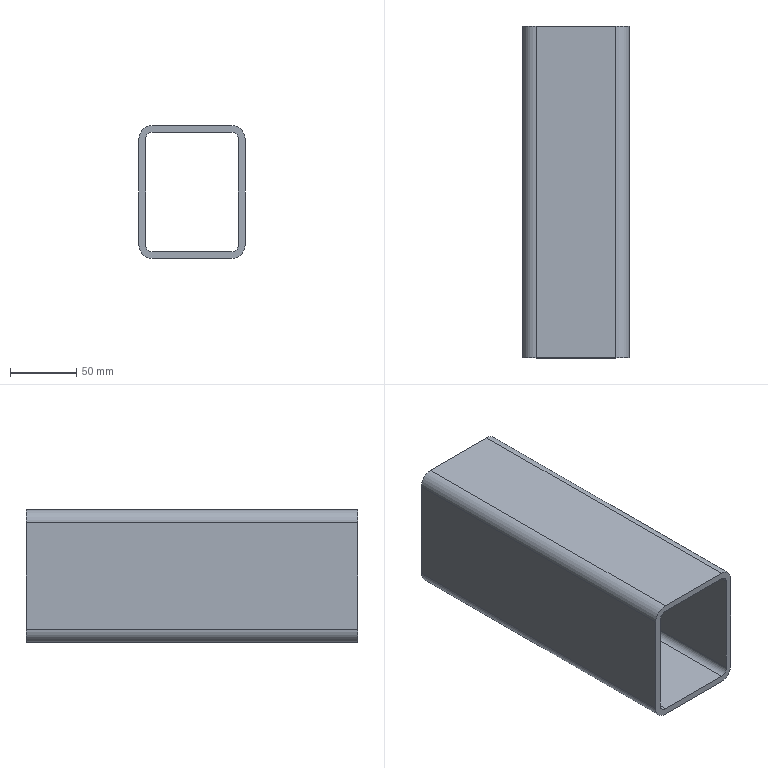Part | SolidWorks | features WeldMemberFeat 1, WeldmentFeature 1 | 1 solid | 18 faces | box 80 x 250 x 100 mm | volume 408905 mm3 | plane 10 | cylinder 8 | commonest cylinder face diameters 10 x4 20 x4
STEP:
#1=CARTESIAN_POINT('',(-40.,0.,40.));
#2=VERTEX_POINT('',#1);
#3=CARTESIAN_POINT('',(-30.,0.,50.));
#4=VERTEX_POINT('',#3);
#5=CARTESIAN_POINT('',(-30.,0.,40.));
#6=DIRECTION('',(0.,1.,0.));
#7=DIRECTION('',(0.,0.,1.));
#8=AXIS2_PLACEMENT_3D('',#5,#6,#7);
#9=CIRCLE('',#8,10.);
#10=EDGE_CURVE('',#2,#4,#9,.T.);
#11=ORIENTED_EDGE('',*,*,#10,.T.);
#12=CARTESIAN_POINT('',(-30.,250.,50.));
#13=VERTEX_POINT('',#12);
#14=CARTESIAN_POINT('',(-30.,250.,50.));
#15=DIRECTION('',(0.,-1.,0.));
#16=VECTOR('',#15,1000.);
#17=LINE('',#14,#16);
#18=EDGE_CURVE('',#13,#4,#17,.T.);
#19=ORIENTED_EDGE('',*,*,#18,.F.);
#20=CARTESIAN_POINT('',(-40.,250.,40.));
#21=VERTEX_POINT('',#20);
#22=CARTESIAN_POINT('',(-30.,250.,40.));
#23=DIRECTION('',(0.,1.,0.));
#24=DIRECTION('',(0.,0.,1.));
#25=AXIS2_PLACEMENT_3D('',#22,#23,#24);
#26=CIRCLE('',#25,10.);
#27=EDGE_CURVE('',#21,#13,#26,.T.);
#28=ORIENTED_EDGE('',*,*,#27,.F.);
#29=CARTESIAN_POINT('',(-40.,250.,40.));
#30=DIRECTION('',(0.,-1.,0.));
#31=VECTOR('',#30,1000.);
#32=LINE('',#29,#31);
#33=EDGE_CURVE('',#21,#2,#32,.T.);
#34=ORIENTED_EDGE('',*,*,#33,.T.);
#35=EDGE_LOOP('',(#11,#19,#28,#34));
#36=FACE_OUTER_BOUND('',#35,.T.);
#37=CARTESIAN_POINT('',(-30.,250.,40.));
#38=DIRECTION('',(0.,-1.,0.));
#39=DIRECTION('',(0.,0.,-1.));
#40=AXIS2_PLACEMENT_3D('',#37,#38,#39);
#41=CYLINDRICAL_SURFACE('',#40,10.);
#42=ADVANCED_FACE('',(#36),#41,.T.);
#43=CARTESIAN_POINT('',(30.,0.,50.));
#44=VERTEX_POINT('',#43);
#45=CARTESIAN_POINT('',(-30.,0.,50.));
#46=DIRECTION('',(1.,0.,0.));
#47=VECTOR('',#46,1000.);
#48=LINE('',#45,#47);
#49=EDGE_CURVE('',#4,#44,#48,.T.);
#50=ORIENTED_EDGE('',*,*,#49,.T.);
#51=CARTESIAN_POINT('',(30.,250.,50.));
#52=VERTEX_POINT('',#51);
#53=CARTESIAN_POINT('',(30.,250.,50.));
#54=DIRECTION('',(0.,-1.,0.));
#55=VECTOR('',#54,1000.);
#56=LINE('',#53,#55);
#57=EDGE_CURVE('',#52,#44,#56,.T.);
#58=ORIENTED_EDGE('',*,*,#57,.F.);
#59=CARTESIAN_POINT('',(-30.,250.,50.));
#60=DIRECTION('',(1.,0.,0.));
#61=VECTOR('',#60,1000.);
#62=LINE('',#59,#61);
#63=EDGE_CURVE('',#13,#52,#62,.T.);
#64=ORIENTED_EDGE('',*,*,#63,.F.);
#65=ORIENTED_EDGE('',*,*,#18,.T.);
#66=EDGE_LOOP('',(#50,#58,#64,#65));
#67=FACE_OUTER_BOUND('',#66,.T.);
#68=CARTESIAN_POINT('',(-30.,250.,50.));
#69=DIRECTION('',(0.,0.,-1.));
#70=DIRECTION('',(-1.,0.,0.));
#71=AXIS2_PLACEMENT_3D('',#68,#69,#70);
#72=PLANE('',#71);
#73=ADVANCED_FACE('',(#67),#72,.F.);
#74=CARTESIAN_POINT('',(40.,0.,40.));
#75=VERTEX_POINT('',#74);
#76=CARTESIAN_POINT('',(30.,0.,40.));
#77=DIRECTION('',(0.,1.,0.));
#78=DIRECTION('',(0.,0.,1.));
#79=AXIS2_PLACEMENT_3D('',#76,#77,#78);
#80=CIRCLE('',#79,10.);
#81=EDGE_CURVE('',#44,#75,#80,.T.);
#82=ORIENTED_EDGE('',*,*,#81,.T.);
#83=CARTESIAN_POINT('',(40.,250.,40.));
#84=VERTEX_POINT('',#83);
#85=CARTESIAN_POINT('',(40.,250.,40.));
#86=DIRECTION('',(0.,-1.,0.));
#87=VECTOR('',#86,1000.);
#88=LINE('',#85,#87);
#89=EDGE_CURVE('',#84,#75,#88,.T.);
#90=ORIENTED_EDGE('',*,*,#89,.F.);
#91=CARTESIAN_POINT('',(30.,250.,40.));
#92=DIRECTION('',(0.,1.,0.));
#93=DIRECTION('',(0.,0.,1.));
#94=AXIS2_PLACEMENT_3D('',#91,#92,#93);
#95=CIRCLE('',#94,10.);
#96=EDGE_CURVE('',#52,#84,#95,.T.);
#97=ORIENTED_EDGE('',*,*,#96,.F.);
#98=ORIENTED_EDGE('',*,*,#57,.T.);
#99=EDGE_LOOP('',(#82,#90,#97,#98));
#100=FACE_OUTER_BOUND('',#99,.T.);
#101=CARTESIAN_POINT('',(30.,250.,40.));
#102=DIRECTION('',(0.,-1.,0.));
#103=DIRECTION('',(0.,0.,-1.));
#104=AXIS2_PLACEMENT_3D('',#101,#102,#103);
#105=CYLINDRICAL_SURFACE('',#104,10.);
#106=ADVANCED_FACE('',(#100),#105,.T.);
#107=CARTESIAN_POINT('',(40.,0.,-40.));
#108=VERTEX_POINT('',#107);
#109=CARTESIAN_POINT('',(40.,0.,-40.));
#110=DIRECTION('',(0.,0.,-1.));
#111=VECTOR('',#110,1000.);
#112=LINE('',#109,#111);
#113=EDGE_CURVE('',#75,#108,#112,.T.);
#114=ORIENTED_EDGE('',*,*,#113,.T.);
#115=CARTESIAN_POINT('',(40.,250.,-40.));
#116=VERTEX_POINT('',#115);
#117=CARTESIAN_POINT('',(40.,250.,-40.));
#118=DIRECTION('',(0.,-1.,0.));
#119=VECTOR('',#118,1000.);
#120=LINE('',#117,#119);
#121=EDGE_CURVE('',#116,#108,#120,.T.);
#122=ORIENTED_EDGE('',*,*,#121,.F.);
#123=CARTESIAN_POINT('',(40.,250.,-40.));
#124=DIRECTION('',(0.,0.,-1.));
#125=VECTOR('',#124,1000.);
#126=LINE('',#123,#125);
#127=EDGE_CURVE('',#84,#116,#126,.T.);
#128=ORIENTED_EDGE('',*,*,#127,.F.);
#129=ORIENTED_EDGE('',*,*,#89,.T.);
#130=EDGE_LOOP('',(#114,#122,#128,#129));
#131=FACE_OUTER_BOUND('',#130,.T.);
#132=CARTESIAN_POINT('',(40.,250.,-40.));
#133=DIRECTION('',(-1.,0.,0.));
#134=DIRECTION('',(0.,0.,1.));
#135=AXIS2_PLACEMENT_3D('',#132,#133,#134);
#136=PLANE('',#135);
#137=ADVANCED_FACE('',(#131),#136,.F.);
#138=CARTESIAN_POINT('',(30.,0.,-50.));
#139=VERTEX_POINT('',#138);
#140=CARTESIAN_POINT('',(30.,0.,-40.));
#141=DIRECTION('',(0.,1.,0.));
#142=DIRECTION('',(0.,0.,1.));
#143=AXIS2_PLACEMENT_3D('',#140,#141,#142);
#144=CIRCLE('',#143,10.);
#145=EDGE_CURVE('',#108,#139,#144,.T.);
#146=ORIENTED_EDGE('',*,*,#145,.T.);
#147=CARTESIAN_POINT('',(30.,250.,-50.));
#148=VERTEX_POINT('',#147);
#149=CARTESIAN_POINT('',(30.,250.,-50.));
#150=DIRECTION('',(0.,-1.,0.));
#151=VECTOR('',#150,1000.);
#152=LINE('',#149,#151);
#153=EDGE_CURVE('',#148,#139,#152,.T.);
#154=ORIENTED_EDGE('',*,*,#153,.F.);
#155=CARTESIAN_POINT('',(30.,250.,-40.));
#156=DIRECTION('',(0.,1.,0.));
#157=DIRECTION('',(0.,0.,1.));
#158=AXIS2_PLACEMENT_3D('',#155,#156,#157);
#159=CIRCLE('',#158,10.);
#160=EDGE_CURVE('',#116,#148,#159,.T.);
#161=ORIENTED_EDGE('',*,*,#160,.F.);
#162=ORIENTED_EDGE('',*,*,#121,.T.);
#163=EDGE_LOOP('',(#146,#154,#161,#162));
#164=FACE_OUTER_BOUND('',#163,.T.);
#165=CARTESIAN_POINT('',(30.,250.,-40.));
#166=DIRECTION('',(0.,-1.,0.));
#167=DIRECTION('',(0.,0.,-1.));
#168=AXIS2_PLACEMENT_3D('',#165,#166,#167);
#169=CYLINDRICAL_SURFACE('',#168,10.);
#170=ADVANCED_FACE('',(#164),#169,.T.);
#171=CARTESIAN_POINT('',(-30.,0.,-50.));
#172=VERTEX_POINT('',#171);
#173=CARTESIAN_POINT('',(30.,0.,-50.));
#174=DIRECTION('',(-1.,0.,0.));
#175=VECTOR('',#174,1000.);
#176=LINE('',#173,#175);
#177=EDGE_CURVE('',#139,#172,#176,.T.);
#178=ORIENTED_EDGE('',*,*,#177,.T.);
#179=CARTESIAN_POINT('',(-30.,250.,-50.));
#180=VERTEX_POINT('',#179);
#181=CARTESIAN_POINT('',(-30.,250.,-50.));
#182=DIRECTION('',(0.,-1.,0.));
#183=VECTOR('',#182,1000.);
#184=LINE('',#181,#183);
#185=EDGE_CURVE('',#180,#172,#184,.T.);
#186=ORIENTED_EDGE('',*,*,#185,.F.);
#187=CARTESIAN_POINT('',(30.,250.,-50.));
#188=DIRECTION('',(-1.,0.,0.));
#189=VECTOR('',#188,1000.);
#190=LINE('',#187,#189);
#191=EDGE_CURVE('',#148,#180,#190,.T.);
#192=ORIENTED_EDGE('',*,*,#191,.F.);
#193=ORIENTED_EDGE('',*,*,#153,.T.);
#194=EDGE_LOOP('',(#178,#186,#192,#193));
#195=FACE_OUTER_BOUND('',#194,.T.);
#196=CARTESIAN_POINT('',(30.,250.,-50.));
#197=DIRECTION('',(0.,0.,1.));
#198=DIRECTION('',(1.,0.,0.));
#199=AXIS2_PLACEMENT_3D('',#196,#197,#198);
#200=PLANE('',#199);
#201=ADVANCED_FACE('',(#195),#200,.F.);
#202=CARTESIAN_POINT('',(-40.,0.,-40.));
#203=VERTEX_POINT('',#202);
#204=CARTESIAN_POINT('',(-30.,0.,-40.));
#205=DIRECTION('',(0.,1.,0.));
#206=DIRECTION('',(0.,0.,1.));
#207=AXIS2_PLACEMENT_3D('',#204,#205,#206);
#208=CIRCLE('',#207,10.);
#209=EDGE_CURVE('',#172,#203,#208,.T.);
#210=ORIENTED_EDGE('',*,*,#209,.T.);
#211=CARTESIAN_POINT('',(-40.,250.,-40.));
#212=VERTEX_POINT('',#211);
#213=CARTESIAN_POINT('',(-40.,250.,-40.));
#214=DIRECTION('',(0.,-1.,0.));
#215=VECTOR('',#214,1000.);
#216=LINE('',#213,#215);
#217=EDGE_CURVE('',#212,#203,#216,.T.);
#218=ORIENTED_EDGE('',*,*,#217,.F.);
#219=CARTESIAN_POINT('',(-30.,250.,-40.));
#220=DIRECTION('',(0.,1.,0.));
#221=DIRECTION('',(0.,0.,1.));
#222=AXIS2_PLACEMENT_3D('',#219,#220,#221);
#223=CIRCLE('',#222,10.);
#224=EDGE_CURVE('',#180,#212,#223,.T.);
#225=ORIENTED_EDGE('',*,*,#224,.F.);
#226=ORIENTED_EDGE('',*,*,#185,.T.);
#227=EDGE_LOOP('',(#210,#218,#225,#226));
#228=FACE_OUTER_BOUND('',#227,.T.);
#229=CARTESIAN_POINT('',(-30.,250.,-40.));
#230=DIRECTION('',(0.,-1.,0.));
#231=DIRECTION('',(0.,0.,-1.));
#232=AXIS2_PLACEMENT_3D('',#229,#230,#231);
#233=CYLINDRICAL_SURFACE('',#232,10.);
#234=ADVANCED_FACE('',(#228),#233,.T.);
#235=CARTESIAN_POINT('',(30.,0.,45.));
#236=VERTEX_POINT('',#235);
#237=CARTESIAN_POINT('',(35.,0.,40.));
#238=VERTEX_POINT('',#237);
#239=CARTESIAN_POINT('',(30.,0.,40.));
#240=DIRECTION('',(0.,1.,0.));
#241=DIRECTION('',(0.,0.,1.));
#242=AXIS2_PLACEMENT_3D('',#239,#240,#241);
#243=CIRCLE('',#242,5.);
#244=EDGE_CURVE('',#236,#238,#243,.T.);
#245=ORIENTED_EDGE('',*,*,#244,.F.);
#246=CARTESIAN_POINT('',(30.,250.,45.));
#247=VERTEX_POINT('',#246);
#248=CARTESIAN_POINT('',(30.,250.,45.));
#249=DIRECTION('',(0.,-1.,0.));
#250=VECTOR('',#249,1000.);
#251=LINE('',#248,#250);
#252=EDGE_CURVE('',#247,#236,#251,.T.);
#253=ORIENTED_EDGE('',*,*,#252,.F.);
#254=CARTESIAN_POINT('',(35.,250.,40.));
#255=VERTEX_POINT('',#254);
#256=CARTESIAN_POINT('',(30.,250.,40.));
#257=DIRECTION('',(0.,1.,0.));
#258=DIRECTION('',(0.,0.,1.));
#259=AXIS2_PLACEMENT_3D('',#256,#257,#258);
#260=CIRCLE('',#259,5.);
#261=EDGE_CURVE('',#247,#255,#260,.T.);
#262=ORIENTED_EDGE('',*,*,#261,.T.);
#263=CARTESIAN_POINT('',(35.,250.,40.));
#264=DIRECTION('',(0.,-1.,0.));
#265=VECTOR('',#264,1000.);
#266=LINE('',#263,#265);
#267=EDGE_CURVE('',#255,#238,#266,.T.);
#268=ORIENTED_EDGE('',*,*,#267,.T.);
#269=EDGE_LOOP('',(#245,#253,#262,#268));
#270=FACE_OUTER_BOUND('',#269,.T.);
#271=CARTESIAN_POINT('',(30.,250.,40.));
#272=DIRECTION('',(0.,-1.,0.));
#273=DIRECTION('',(0.,0.,-1.));
#274=AXIS2_PLACEMENT_3D('',#271,#272,#273);
#275=CYLINDRICAL_SURFACE('',#274,5.);
#276=ADVANCED_FACE('',(#270),#275,.F.);
#277=CARTESIAN_POINT('',(-30.,0.,45.));
#278=VERTEX_POINT('',#277);
#279=CARTESIAN_POINT('',(-30.,0.,45.));
#280=DIRECTION('',(1.,0.,0.));
#281=VECTOR('',#280,1000.);
#282=LINE('',#279,#281);
#283=EDGE_CURVE('',#278,#236,#282,.T.);
#284=ORIENTED_EDGE('',*,*,#283,.F.);
#285=CARTESIAN_POINT('',(-30.,250.,45.));
#286=VERTEX_POINT('',#285);
#287=CARTESIAN_POINT('',(-30.,250.,45.));
#288=DIRECTION('',(0.,-1.,0.));
#289=VECTOR('',#288,1000.);
#290=LINE('',#287,#289);
#291=EDGE_CURVE('',#286,#278,#290,.T.);
#292=ORIENTED_EDGE('',*,*,#291,.F.);
#293=CARTESIAN_POINT('',(-30.,250.,45.));
#294=DIRECTION('',(1.,0.,0.));
#295=VECTOR('',#294,1000.);
#296=LINE('',#293,#295);
#297=EDGE_CURVE('',#286,#247,#296,.T.);
#298=ORIENTED_EDGE('',*,*,#297,.T.);
#299=ORIENTED_EDGE('',*,*,#252,.T.);
#300=EDGE_LOOP('',(#284,#292,#298,#299));
#301=FACE_OUTER_BOUND('',#300,.T.);
#302=CARTESIAN_POINT('',(-30.,250.,45.));
#303=DIRECTION('',(0.,0.,-1.));
#304=DIRECTION('',(-1.,0.,0.));
#305=AXIS2_PLACEMENT_3D('',#302,#303,#304);
#306=PLANE('',#305);
#307=ADVANCED_FACE('',(#301),#306,.T.);
#308=CARTESIAN_POINT('',(-35.,0.,40.));
#309=VERTEX_POINT('',#308);
#310=CARTESIAN_POINT('',(-30.,0.,40.));
#311=DIRECTION('',(0.,1.,0.));
#312=DIRECTION('',(0.,0.,1.));
#313=AXIS2_PLACEMENT_3D('',#310,#311,#312);
#314=CIRCLE('',#313,5.);
#315=EDGE_CURVE('',#309,#278,#314,.T.);
#316=ORIENTED_EDGE('',*,*,#315,.F.);
#317=CARTESIAN_POINT('',(-35.,250.,40.));
#318=VERTEX_POINT('',#317);
#319=CARTESIAN_POINT('',(-35.,250.,40.));
#320=DIRECTION('',(0.,-1.,0.));
#321=VECTOR('',#320,1000.);
#322=LINE('',#319,#321);
#323=EDGE_CURVE('',#318,#309,#322,.T.);
#324=ORIENTED_EDGE('',*,*,#323,.F.);
#325=CARTESIAN_POINT('',(-30.,250.,40.));
#326=DIRECTION('',(0.,1.,0.));
#327=DIRECTION('',(0.,0.,1.));
#328=AXIS2_PLACEMENT_3D('',#325,#326,#327);
#329=CIRCLE('',#328,5.);
#330=EDGE_CURVE('',#318,#286,#329,.T.);
#331=ORIENTED_EDGE('',*,*,#330,.T.);
#332=ORIENTED_EDGE('',*,*,#291,.T.);
#333=EDGE_LOOP('',(#316,#324,#331,#332));
#334=FACE_OUTER_BOUND('',#333,.T.);
#335=CARTESIAN_POINT('',(-30.,250.,40.));
#336=DIRECTION('',(0.,-1.,0.));
#337=DIRECTION('',(0.,0.,-1.));
#338=AXIS2_PLACEMENT_3D('',#335,#336,#337);
#339=CYLINDRICAL_SURFACE('',#338,5.);
#340=ADVANCED_FACE('',(#334),#339,.F.);
#341=CARTESIAN_POINT('',(-35.,0.,-40.));
#342=VERTEX_POINT('',#341);
#343=CARTESIAN_POINT('',(-35.,0.,40.));
#344=DIRECTION('',(0.,0.,1.));
#345=VECTOR('',#344,1000.);
#346=LINE('',#343,#345);
#347=EDGE_CURVE('',#342,#309,#346,.T.);
#348=ORIENTED_EDGE('',*,*,#347,.F.);
#349=CARTESIAN_POINT('',(-35.,250.,-40.));
#350=VERTEX_POINT('',#349);
#351=CARTESIAN_POINT('',(-35.,250.,-40.));
#352=DIRECTION('',(0.,-1.,0.));
#353=VECTOR('',#352,1000.);
#354=LINE('',#351,#353);
#355=EDGE_CURVE('',#350,#342,#354,.T.);
#356=ORIENTED_EDGE('',*,*,#355,.F.);
#357=CARTESIAN_POINT('',(-35.,250.,40.));
#358=DIRECTION('',(0.,0.,1.));
#359=VECTOR('',#358,1000.);
#360=LINE('',#357,#359);
#361=EDGE_CURVE('',#350,#318,#360,.T.);
#362=ORIENTED_EDGE('',*,*,#361,.T.);
#363=ORIENTED_EDGE('',*,*,#323,.T.);
#364=EDGE_LOOP('',(#348,#356,#362,#363));
#365=FACE_OUTER_BOUND('',#364,.T.);
#366=CARTESIAN_POINT('',(-35.,250.,40.));
#367=DIRECTION('',(1.,0.,0.));
#368=DIRECTION('',(0.,0.,-1.));
#369=AXIS2_PLACEMENT_3D('',#366,#367,#368);
#370=PLANE('',#369);
#371=ADVANCED_FACE('',(#365),#370,.T.);
#372=CARTESIAN_POINT('',(-30.,0.,-45.));
#373=VERTEX_POINT('',#372);
#374=CARTESIAN_POINT('',(-30.,0.,-40.));
#375=DIRECTION('',(0.,1.,0.));
#376=DIRECTION('',(0.,0.,1.));
#377=AXIS2_PLACEMENT_3D('',#374,#375,#376);
#378=CIRCLE('',#377,5.);
#379=EDGE_CURVE('',#373,#342,#378,.T.);
#380=ORIENTED_EDGE('',*,*,#379,.F.);
#381=CARTESIAN_POINT('',(-30.,250.,-45.));
#382=VERTEX_POINT('',#381);
#383=CARTESIAN_POINT('',(-30.,250.,-45.));
#384=DIRECTION('',(0.,-1.,0.));
#385=VECTOR('',#384,1000.);
#386=LINE('',#383,#385);
#387=EDGE_CURVE('',#382,#373,#386,.T.);
#388=ORIENTED_EDGE('',*,*,#387,.F.);
#389=CARTESIAN_POINT('',(-30.,250.,-40.));
#390=DIRECTION('',(0.,1.,0.));
#391=DIRECTION('',(0.,0.,1.));
#392=AXIS2_PLACEMENT_3D('',#389,#390,#391);
#393=CIRCLE('',#392,5.);
#394=EDGE_CURVE('',#382,#350,#393,.T.);
#395=ORIENTED_EDGE('',*,*,#394,.T.);
#396=ORIENTED_EDGE('',*,*,#355,.T.);
#397=EDGE_LOOP('',(#380,#388,#395,#396));
#398=FACE_OUTER_BOUND('',#397,.T.);
#399=CARTESIAN_POINT('',(-30.,250.,-40.));
#400=DIRECTION('',(0.,-1.,0.));
#401=DIRECTION('',(0.,0.,-1.));
#402=AXIS2_PLACEMENT_3D('',#399,#400,#401);
#403=CYLINDRICAL_SURFACE('',#402,5.);
#404=ADVANCED_FACE('',(#398),#403,.F.);
#405=CARTESIAN_POINT('',(30.,0.,-45.));
#406=VERTEX_POINT('',#405);
#407=CARTESIAN_POINT('',(30.,0.,-45.));
#408=DIRECTION('',(-1.,0.,0.));
#409=VECTOR('',#408,1000.);
#410=LINE('',#407,#409);
#411=EDGE_CURVE('',#406,#373,#410,.T.);
#412=ORIENTED_EDGE('',*,*,#411,.F.);
#413=CARTESIAN_POINT('',(30.,250.,-45.));
#414=VERTEX_POINT('',#413);
#415=CARTESIAN_POINT('',(30.,250.,-45.));
#416=DIRECTION('',(0.,-1.,0.));
#417=VECTOR('',#416,1000.);
#418=LINE('',#415,#417);
#419=EDGE_CURVE('',#414,#406,#418,.T.);
#420=ORIENTED_EDGE('',*,*,#419,.F.);
#421=CARTESIAN_POINT('',(30.,250.,-45.));
#422=DIRECTION('',(-1.,0.,0.));
#423=VECTOR('',#422,1000.);
#424=LINE('',#421,#423);
#425=EDGE_CURVE('',#414,#382,#424,.T.);
#426=ORIENTED_EDGE('',*,*,#425,.T.);
#427=ORIENTED_EDGE('',*,*,#387,.T.);
#428=EDGE_LOOP('',(#412,#420,#426,#427));
#429=FACE_OUTER_BOUND('',#428,.T.);
#430=CARTESIAN_POINT('',(30.,250.,-45.));
#431=DIRECTION('',(0.,0.,1.));
#432=DIRECTION('',(1.,0.,0.));
#433=AXIS2_PLACEMENT_3D('',#430,#431,#432);
#434=PLANE('',#433);
#435=ADVANCED_FACE('',(#429),#434,.T.);
#436=CARTESIAN_POINT('',(35.,0.,-40.));
#437=VERTEX_POINT('',#436);
#438=CARTESIAN_POINT('',(30.,0.,-40.));
#439=DIRECTION('',(0.,1.,0.));
#440=DIRECTION('',(0.,0.,1.));
#441=AXIS2_PLACEMENT_3D('',#438,#439,#440);
#442=CIRCLE('',#441,5.);
#443=EDGE_CURVE('',#437,#406,#442,.T.);
#444=ORIENTED_EDGE('',*,*,#443,.F.);
#445=CARTESIAN_POINT('',(35.,250.,-40.));
#446=VERTEX_POINT('',#445);
#447=CARTESIAN_POINT('',(35.,250.,-40.));
#448=DIRECTION('',(0.,-1.,0.));
#449=VECTOR('',#448,1000.);
#450=LINE('',#447,#449);
#451=EDGE_CURVE('',#446,#437,#450,.T.);
#452=ORIENTED_EDGE('',*,*,#451,.F.);
#453=CARTESIAN_POINT('',(30.,250.,-40.));
#454=DIRECTION('',(0.,1.,0.));
#455=DIRECTION('',(0.,0.,1.));
#456=AXIS2_PLACEMENT_3D('',#453,#454,#455);
#457=CIRCLE('',#456,5.);
#458=EDGE_CURVE('',#446,#414,#457,.T.);
#459=ORIENTED_EDGE('',*,*,#458,.T.);
#460=ORIENTED_EDGE('',*,*,#419,.T.);
#461=EDGE_LOOP('',(#444,#452,#459,#460));
#462=FACE_OUTER_BOUND('',#461,.T.);
#463=CARTESIAN_POINT('',(30.,250.,-40.));
#464=DIRECTION('',(0.,-1.,0.));
#465=DIRECTION('',(0.,0.,-1.));
#466=AXIS2_PLACEMENT_3D('',#463,#464,#465);
#467=CYLINDRICAL_SURFACE('',#466,5.);
#468=ADVANCED_FACE('',(#462),#467,.F.);
#469=CARTESIAN_POINT('',(35.,0.,-40.));
#470=DIRECTION('',(0.,0.,-1.));
#471=VECTOR('',#470,1000.);
#472=LINE('',#469,#471);
#473=EDGE_CURVE('',#238,#437,#472,.T.);
#474=ORIENTED_EDGE('',*,*,#473,.F.);
#475=ORIENTED_EDGE('',*,*,#267,.F.);
#476=CARTESIAN_POINT('',(35.,250.,-40.));
#477=DIRECTION('',(0.,0.,-1.));
#478=VECTOR('',#477,1000.);
#479=LINE('',#476,#478);
#480=EDGE_CURVE('',#255,#446,#479,.T.);
#481=ORIENTED_EDGE('',*,*,#480,.T.);
#482=ORIENTED_EDGE('',*,*,#451,.T.);
#483=EDGE_LOOP('',(#474,#475,#481,#482));
#484=FACE_OUTER_BOUND('',#483,.T.);
#485=CARTESIAN_POINT('',(35.,250.,-40.));
#486=DIRECTION('',(-1.,0.,0.));
#487=DIRECTION('',(0.,0.,1.));
#488=AXIS2_PLACEMENT_3D('',#485,#486,#487);
#489=PLANE('',#488);
#490=ADVANCED_FACE('',(#484),#489,.T.);
#491=CARTESIAN_POINT('',(-40.,0.,40.));
#492=DIRECTION('',(0.,0.,1.));
#493=VECTOR('',#492,1000.);
#494=LINE('',#491,#493);
#495=EDGE_CURVE('',#203,#2,#494,.T.);
#496=ORIENTED_EDGE('',*,*,#495,.T.);
#497=ORIENTED_EDGE('',*,*,#33,.F.);
#498=CARTESIAN_POINT('',(-40.,250.,40.));
#499=DIRECTION('',(0.,0.,1.));
#500=VECTOR('',#499,1000.);
#501=LINE('',#498,#500);
#502=EDGE_CURVE('',#212,#21,#501,.T.);
#503=ORIENTED_EDGE('',*,*,#502,.F.);
#504=ORIENTED_EDGE('',*,*,#217,.T.);
#505=EDGE_LOOP('',(#496,#497,#503,#504));
#506=FACE_OUTER_BOUND('',#505,.T.);
#507=CARTESIAN_POINT('',(-40.,250.,40.));
#508=DIRECTION('',(1.,0.,0.));
#509=DIRECTION('',(0.,0.,-1.));
#510=AXIS2_PLACEMENT_3D('',#507,#508,#509);
#511=PLANE('',#510);
#512=ADVANCED_FACE('',(#506),#511,.F.);
#513=ORIENTED_EDGE('',*,*,#261,.F.);
#514=ORIENTED_EDGE('',*,*,#297,.F.);
#515=ORIENTED_EDGE('',*,*,#330,.F.);
#516=ORIENTED_EDGE('',*,*,#361,.F.);
#517=ORIENTED_EDGE('',*,*,#394,.F.);
#518=ORIENTED_EDGE('',*,*,#425,.F.);
#519=ORIENTED_EDGE('',*,*,#458,.F.);
#520=ORIENTED_EDGE('',*,*,#480,.F.);
#521=EDGE_LOOP('',(#513,#514,#515,#516,#517,#518,#519,#520));
#522=FACE_BOUND('',#521,.T.);
#523=ORIENTED_EDGE('',*,*,#27,.T.);
#524=ORIENTED_EDGE('',*,*,#63,.T.);
#525=ORIENTED_EDGE('',*,*,#96,.T.);
#526=ORIENTED_EDGE('',*,*,#127,.T.);
#527=ORIENTED_EDGE('',*,*,#160,.T.);
#528=ORIENTED_EDGE('',*,*,#191,.T.);
#529=ORIENTED_EDGE('',*,*,#224,.T.);
#530=ORIENTED_EDGE('',*,*,#502,.T.);
#531=EDGE_LOOP('',(#523,#524,#525,#526,#527,#528,#529,#530));
#532=FACE_OUTER_BOUND('',#531,.T.);
#533=CARTESIAN_POINT('',(-30.,250.,40.));
#534=DIRECTION('',(0.,1.,0.));
#535=DIRECTION('',(0.,0.,1.));
#536=AXIS2_PLACEMENT_3D('',#533,#534,#535);
#537=PLANE('',#536);
#538=ADVANCED_FACE('',(#522,#532),#537,.T.);
#539=ORIENTED_EDGE('',*,*,#244,.T.);
#540=ORIENTED_EDGE('',*,*,#473,.T.);
#541=ORIENTED_EDGE('',*,*,#443,.T.);
#542=ORIENTED_EDGE('',*,*,#411,.T.);
#543=ORIENTED_EDGE('',*,*,#379,.T.);
#544=ORIENTED_EDGE('',*,*,#347,.T.);
#545=ORIENTED_EDGE('',*,*,#315,.T.);
#546=ORIENTED_EDGE('',*,*,#283,.T.);
#547=EDGE_LOOP('',(#539,#540,#541,#542,#543,#544,#545,#546));
#548=FACE_BOUND('',#547,.T.);
#549=ORIENTED_EDGE('',*,*,#10,.F.);
#550=ORIENTED_EDGE('',*,*,#495,.F.);
#551=ORIENTED_EDGE('',*,*,#209,.F.);
#552=ORIENTED_EDGE('',*,*,#177,.F.);
#553=ORIENTED_EDGE('',*,*,#145,.F.);
#554=ORIENTED_EDGE('',*,*,#113,.F.);
#555=ORIENTED_EDGE('',*,*,#81,.F.);
#556=ORIENTED_EDGE('',*,*,#49,.F.);
#557=EDGE_LOOP('',(#549,#550,#551,#552,#553,#554,#555,#556));
#558=FACE_OUTER_BOUND('',#557,.T.);
#559=CARTESIAN_POINT('',(-30.,0.,40.));
#560=DIRECTION('',(0.,1.,0.));
#561=DIRECTION('',(0.,0.,1.));
#562=AXIS2_PLACEMENT_3D('',#559,#560,#561);
#563=PLANE('',#562);
#564=ADVANCED_FACE('',(#548,#558),#563,.F.);
#565=CLOSED_SHELL('',(#42,#73,#106,#137,#170,#201,#234,#276,#307,#340,#371,#404,#435,#468,#490,#512,#538,#564));
#566=MANIFOLD_SOLID_BREP('',#565);
#567=CARTESIAN_POINT('',(0.,0.,0.));
#568=DIRECTION('',(0.,0.,1.));
#569=DIRECTION('',(1.,0.,0.));
#570=AXIS2_PLACEMENT_3D('',#567,#568,#569);
#571=(LENGTH_UNIT()NAMED_UNIT(*)SI_UNIT(.MILLI.,.METRE.));
#572=UNCERTAINTY_MEASURE_WITH_UNIT(LENGTH_MEASURE(0.00001),#571,'','');
#573=(NAMED_UNIT(*)PLANE_ANGLE_UNIT()SI_UNIT($,.RADIAN.));
#574=(NAMED_UNIT(*)SI_UNIT($,.STERADIAN.)SOLID_ANGLE_UNIT());
#575=(GEOMETRIC_REPRESENTATION_CONTEXT(3)GLOBAL_UNCERTAINTY_ASSIGNED_CONTEXT((#572))GLOBAL_UNIT_ASSIGNED_CONTEXT((#571,#573,#574))REPRESENTATION_CONTEXT('',''));
#576=ADVANCED_BREP_SHAPE_REPRESENTATION('',(#566,#570),#575);